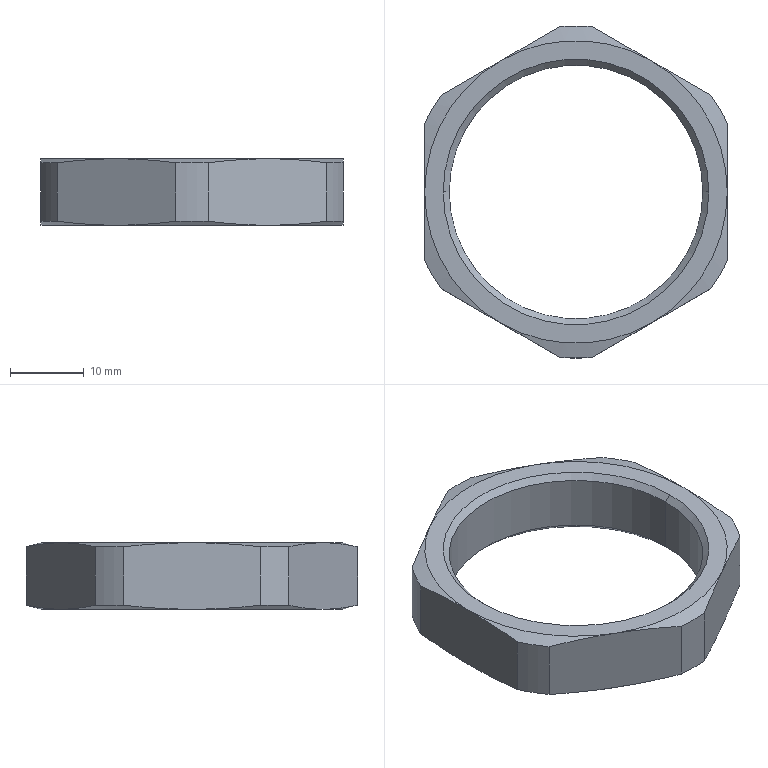Part | SolidWorks | features BaseBody 1 | 1 solid | 32 faces | box 41 x 45 x 9 mm | volume 4491 mm3 | cone 16 | cylinder 8 | plane 8 | commonest cylinder face diameters 45 x6 34.376 x2
STEP:
#1=CARTESIAN_POINT('',(-17.188,0.,0.812));
#2=VERTEX_POINT('',#1);
#3=CARTESIAN_POINT('',(17.188,0.,0.812));
#4=VERTEX_POINT('',#3);
#5=CARTESIAN_POINT('',(0.,0.,0.812));
#6=DIRECTION('',(0.,0.,1.));
#7=DIRECTION('',(1.,0.,0.));
#8=AXIS2_PLACEMENT_3D('',#5,#6,#7);
#9=CIRCLE('',#8,17.188);
#10=EDGE_CURVE('',#2,#4,#9,.T.);
#11=ORIENTED_EDGE('',*,*,#10,.F.);
#12=CARTESIAN_POINT('',(-17.188,0.,8.188));
#13=VERTEX_POINT('',#12);
#14=CARTESIAN_POINT('',(-17.188,0.,0.));
#15=DIRECTION('',(0.,0.,1.));
#16=VECTOR('',#15,1000.);
#17=LINE('',#14,#16);
#18=EDGE_CURVE('',#2,#13,#17,.T.);
#19=ORIENTED_EDGE('',*,*,#18,.T.);
#20=CARTESIAN_POINT('',(17.188,0.,8.188));
#21=VERTEX_POINT('',#20);
#22=CARTESIAN_POINT('',(0.,0.,8.188));
#23=DIRECTION('',(0.,0.,-1.));
#24=DIRECTION('',(1.,0.,0.));
#25=AXIS2_PLACEMENT_3D('',#22,#23,#24);
#26=CIRCLE('',#25,17.188);
#27=EDGE_CURVE('',#21,#13,#26,.T.);
#28=ORIENTED_EDGE('',*,*,#27,.F.);
#29=CARTESIAN_POINT('',(17.188,0.,0.));
#30=DIRECTION('',(0.,0.,1.));
#31=VECTOR('',#30,1000.);
#32=LINE('',#29,#31);
#33=EDGE_CURVE('',#4,#21,#32,.T.);
#34=ORIENTED_EDGE('',*,*,#33,.F.);
#35=EDGE_LOOP('',(#11,#19,#28,#34));
#36=FACE_OUTER_BOUND('',#35,.T.);
#37=CARTESIAN_POINT('',(0.,0.,0.));
#38=DIRECTION('',(0.,0.,1.));
#39=DIRECTION('',(1.,0.,0.));
#40=AXIS2_PLACEMENT_3D('',#37,#38,#39);
#41=CYLINDRICAL_SURFACE('',#40,17.188);
#42=ADVANCED_FACE('',(#36),#41,.F.);
#43=ORIENTED_EDGE('',*,*,#27,.T.);
#44=CARTESIAN_POINT('',(-18.,0.,9.));
#45=VERTEX_POINT('',#44);
#46=CARTESIAN_POINT('',(-18.,0.,9.));
#47=DIRECTION('',(-0.7071,0.,0.7071));
#48=VECTOR('',#47,1000.);
#49=LINE('',#46,#48);
#50=EDGE_CURVE('',#13,#45,#49,.T.);
#51=ORIENTED_EDGE('',*,*,#50,.T.);
#52=CARTESIAN_POINT('',(18.,0.,9.));
#53=VERTEX_POINT('',#52);
#54=CARTESIAN_POINT('',(0.,0.,9.));
#55=DIRECTION('',(0.,0.,-1.));
#56=DIRECTION('',(1.,0.,0.));
#57=AXIS2_PLACEMENT_3D('',#54,#55,#56);
#58=CIRCLE('',#57,18.);
#59=EDGE_CURVE('',#53,#45,#58,.T.);
#60=ORIENTED_EDGE('',*,*,#59,.F.);
#61=CARTESIAN_POINT('',(18.,0.,9.));
#62=DIRECTION('',(0.7071,0.,0.7071));
#63=VECTOR('',#62,1000.);
#64=LINE('',#61,#63);
#65=EDGE_CURVE('',#21,#53,#64,.T.);
#66=ORIENTED_EDGE('',*,*,#65,.F.);
#67=EDGE_LOOP('',(#43,#51,#60,#66));
#68=FACE_OUTER_BOUND('',#67,.T.);
#69=CARTESIAN_POINT('',(0.,0.,9.));
#70=DIRECTION('',(0.,0.,1.));
#71=DIRECTION('',(1.,0.,0.));
#72=AXIS2_PLACEMENT_3D('',#69,#70,#71);
#73=CONICAL_SURFACE('',#72,18.,0.7854);
#74=ADVANCED_FACE('',(#68),#73,.F.);
#75=ORIENTED_EDGE('',*,*,#10,.T.);
#76=CARTESIAN_POINT('',(18.,0.,0.));
#77=VERTEX_POINT('',#76);
#78=CARTESIAN_POINT('',(18.,0.,0.));
#79=DIRECTION('',(0.7071,0.,-0.7071));
#80=VECTOR('',#79,1000.);
#81=LINE('',#78,#80);
#82=EDGE_CURVE('',#4,#77,#81,.T.);
#83=ORIENTED_EDGE('',*,*,#82,.T.);
#84=CARTESIAN_POINT('',(-18.,0.,0.));
#85=VERTEX_POINT('',#84);
#86=CARTESIAN_POINT('',(0.,0.,0.));
#87=DIRECTION('',(0.,0.,1.));
#88=DIRECTION('',(-1.,0.,0.));
#89=AXIS2_PLACEMENT_3D('',#86,#87,#88);
#90=CIRCLE('',#89,18.);
#91=EDGE_CURVE('',#85,#77,#90,.T.);
#92=ORIENTED_EDGE('',*,*,#91,.F.);
#93=CARTESIAN_POINT('',(-18.,0.,0.));
#94=DIRECTION('',(-0.7071,0.,-0.7071));
#95=VECTOR('',#94,1000.);
#96=LINE('',#93,#95);
#97=EDGE_CURVE('',#2,#85,#96,.T.);
#98=ORIENTED_EDGE('',*,*,#97,.F.);
#99=EDGE_LOOP('',(#75,#83,#92,#98));
#100=FACE_OUTER_BOUND('',#99,.T.);
#101=CARTESIAN_POINT('',(0.,0.,0.));
#102=DIRECTION('',(0.,0.,-1.));
#103=DIRECTION('',(-1.,0.,0.));
#104=AXIS2_PLACEMENT_3D('',#101,#102,#103);
#105=CONICAL_SURFACE('',#104,18.,0.7854);
#106=ADVANCED_FACE('',(#100),#105,.F.);
#107=ORIENTED_EDGE('',*,*,#18,.F.);
#108=CARTESIAN_POINT('',(0.,0.,0.812));
#109=DIRECTION('',(0.,0.,1.));
#110=DIRECTION('',(1.,0.,0.));
#111=AXIS2_PLACEMENT_3D('',#108,#109,#110);
#112=CIRCLE('',#111,17.188);
#113=EDGE_CURVE('',#4,#2,#112,.T.);
#114=ORIENTED_EDGE('',*,*,#113,.F.);
#115=ORIENTED_EDGE('',*,*,#33,.T.);
#116=CARTESIAN_POINT('',(0.,0.,8.188));
#117=DIRECTION('',(0.,0.,-1.));
#118=DIRECTION('',(1.,0.,0.));
#119=AXIS2_PLACEMENT_3D('',#116,#117,#118);
#120=CIRCLE('',#119,17.188);
#121=EDGE_CURVE('',#13,#21,#120,.T.);
#122=ORIENTED_EDGE('',*,*,#121,.F.);
#123=EDGE_LOOP('',(#107,#114,#115,#122));
#124=FACE_OUTER_BOUND('',#123,.T.);
#125=CARTESIAN_POINT('',(0.,0.,0.));
#126=DIRECTION('',(0.,0.,1.));
#127=DIRECTION('',(1.,0.,0.));
#128=AXIS2_PLACEMENT_3D('',#125,#126,#127);
#129=CYLINDRICAL_SURFACE('',#128,17.188);
#130=ADVANCED_FACE('',(#124),#129,.F.);
#131=ORIENTED_EDGE('',*,*,#50,.F.);
#132=ORIENTED_EDGE('',*,*,#121,.T.);
#133=ORIENTED_EDGE('',*,*,#65,.T.);
#134=CARTESIAN_POINT('',(0.,0.,9.));
#135=DIRECTION('',(0.,0.,-1.));
#136=DIRECTION('',(1.,0.,0.));
#137=AXIS2_PLACEMENT_3D('',#134,#135,#136);
#138=CIRCLE('',#137,18.);
#139=EDGE_CURVE('',#45,#53,#138,.T.);
#140=ORIENTED_EDGE('',*,*,#139,.F.);
#141=EDGE_LOOP('',(#131,#132,#133,#140));
#142=FACE_OUTER_BOUND('',#141,.T.);
#143=CARTESIAN_POINT('',(0.,0.,9.));
#144=DIRECTION('',(0.,0.,1.));
#145=DIRECTION('',(1.,0.,0.));
#146=AXIS2_PLACEMENT_3D('',#143,#144,#145);
#147=CONICAL_SURFACE('',#146,18.,0.7854);
#148=ADVANCED_FACE('',(#142),#147,.F.);
#149=ORIENTED_EDGE('',*,*,#82,.F.);
#150=ORIENTED_EDGE('',*,*,#113,.T.);
#151=ORIENTED_EDGE('',*,*,#97,.T.);
#152=CARTESIAN_POINT('',(0.,0.,0.));
#153=DIRECTION('',(0.,0.,1.));
#154=DIRECTION('',(-1.,0.,0.));
#155=AXIS2_PLACEMENT_3D('',#152,#153,#154);
#156=CIRCLE('',#155,18.);
#157=EDGE_CURVE('',#77,#85,#156,.T.);
#158=ORIENTED_EDGE('',*,*,#157,.F.);
#159=EDGE_LOOP('',(#149,#150,#151,#158));
#160=FACE_OUTER_BOUND('',#159,.T.);
#161=CARTESIAN_POINT('',(0.,0.,0.));
#162=DIRECTION('',(0.,0.,-1.));
#163=DIRECTION('',(-1.,0.,0.));
#164=AXIS2_PLACEMENT_3D('',#161,#162,#163);
#165=CONICAL_SURFACE('',#164,18.,0.7854);
#166=ADVANCED_FACE('',(#160),#165,.F.);
#167=CARTESIAN_POINT('',(10.25,-17.754,9.));
#168=VERTEX_POINT('',#167);
#169=CARTESIAN_POINT('',(20.5,0.,9.));
#170=VERTEX_POINT('',#169);
#171=CARTESIAN_POINT('',(0.,0.,9.));
#172=DIRECTION('',(0.,0.,1.));
#173=DIRECTION('',(-1.,0.,0.));
#174=AXIS2_PLACEMENT_3D('',#171,#172,#173);
#175=CIRCLE('',#174,20.5);
#176=EDGE_CURVE('',#168,#170,#175,.T.);
#177=ORIENTED_EDGE('',*,*,#176,.T.);
#178=CARTESIAN_POINT('',(10.25,17.754,9.));
#179=VERTEX_POINT('',#178);
#180=CARTESIAN_POINT('',(0.,0.,9.));
#181=DIRECTION('',(0.,0.,1.));
#182=DIRECTION('',(-1.,0.,0.));
#183=AXIS2_PLACEMENT_3D('',#180,#181,#182);
#184=CIRCLE('',#183,20.5);
#185=EDGE_CURVE('',#170,#179,#184,.T.);
#186=ORIENTED_EDGE('',*,*,#185,.T.);
#187=CARTESIAN_POINT('',(-10.25,17.754,9.));
#188=VERTEX_POINT('',#187);
#189=CARTESIAN_POINT('',(0.,0.,9.));
#190=DIRECTION('',(0.,0.,1.));
#191=DIRECTION('',(-1.,0.,0.));
#192=AXIS2_PLACEMENT_3D('',#189,#190,#191);
#193=CIRCLE('',#192,20.5);
#194=EDGE_CURVE('',#179,#188,#193,.T.);
#195=ORIENTED_EDGE('',*,*,#194,.T.);
#196=CARTESIAN_POINT('',(-20.5,0.,9.));
#197=VERTEX_POINT('',#196);
#198=CARTESIAN_POINT('',(0.,0.,9.));
#199=DIRECTION('',(0.,0.,1.));
#200=DIRECTION('',(-1.,0.,0.));
#201=AXIS2_PLACEMENT_3D('',#198,#199,#200);
#202=CIRCLE('',#201,20.5);
#203=EDGE_CURVE('',#188,#197,#202,.T.);
#204=ORIENTED_EDGE('',*,*,#203,.T.);
#205=CARTESIAN_POINT('',(-10.25,-17.754,9.));
#206=VERTEX_POINT('',#205);
#207=CARTESIAN_POINT('',(0.,0.,9.));
#208=DIRECTION('',(0.,0.,1.));
#209=DIRECTION('',(-1.,0.,0.));
#210=AXIS2_PLACEMENT_3D('',#207,#208,#209);
#211=CIRCLE('',#210,20.5);
#212=EDGE_CURVE('',#197,#206,#211,.T.);
#213=ORIENTED_EDGE('',*,*,#212,.T.);
#214=CARTESIAN_POINT('',(0.,0.,9.));
#215=DIRECTION('',(0.,0.,1.));
#216=DIRECTION('',(-1.,0.,0.));
#217=AXIS2_PLACEMENT_3D('',#214,#215,#216);
#218=CIRCLE('',#217,20.5);
#219=EDGE_CURVE('',#206,#168,#218,.T.);
#220=ORIENTED_EDGE('',*,*,#219,.T.);
#221=EDGE_LOOP('',(#177,#186,#195,#204,#213,#220));
#222=FACE_OUTER_BOUND('',#221,.T.);
#223=ORIENTED_EDGE('',*,*,#59,.T.);
#224=ORIENTED_EDGE('',*,*,#139,.T.);
#225=EDGE_LOOP('',(#223,#224));
#226=FACE_BOUND('',#225,.T.);
#227=CARTESIAN_POINT('',(0.,20.5,9.));
#228=DIRECTION('',(0.,0.,1.));
#229=DIRECTION('',(1.,0.,0.));
#230=AXIS2_PLACEMENT_3D('',#227,#228,#229);
#231=PLANE('',#230);
#232=ADVANCED_FACE('',(#222,#226),#231,.T.);
#233=ORIENTED_EDGE('',*,*,#91,.T.);
#234=ORIENTED_EDGE('',*,*,#157,.T.);
#235=EDGE_LOOP('',(#233,#234));
#236=FACE_BOUND('',#235,.T.);
#237=CARTESIAN_POINT('',(10.25,-17.754,0.));
#238=VERTEX_POINT('',#237);
#239=CARTESIAN_POINT('',(-10.25,-17.754,0.));
#240=VERTEX_POINT('',#239);
#241=CARTESIAN_POINT('',(0.,0.,0.));
#242=DIRECTION('',(0.,0.,-1.));
#243=DIRECTION('',(1.,0.,0.));
#244=AXIS2_PLACEMENT_3D('',#241,#242,#243);
#245=CIRCLE('',#244,20.5);
#246=EDGE_CURVE('',#238,#240,#245,.T.);
#247=ORIENTED_EDGE('',*,*,#246,.T.);
#248=CARTESIAN_POINT('',(-20.5,0.,0.));
#249=VERTEX_POINT('',#248);
#250=CARTESIAN_POINT('',(0.,0.,0.));
#251=DIRECTION('',(0.,0.,-1.));
#252=DIRECTION('',(1.,0.,0.));
#253=AXIS2_PLACEMENT_3D('',#250,#251,#252);
#254=CIRCLE('',#253,20.5);
#255=EDGE_CURVE('',#240,#249,#254,.T.);
#256=ORIENTED_EDGE('',*,*,#255,.T.);
#257=CARTESIAN_POINT('',(-10.25,17.754,0.));
#258=VERTEX_POINT('',#257);
#259=CARTESIAN_POINT('',(0.,0.,0.));
#260=DIRECTION('',(0.,0.,-1.));
#261=DIRECTION('',(1.,0.,0.));
#262=AXIS2_PLACEMENT_3D('',#259,#260,#261);
#263=CIRCLE('',#262,20.5);
#264=EDGE_CURVE('',#249,#258,#263,.T.);
#265=ORIENTED_EDGE('',*,*,#264,.T.);
#266=CARTESIAN_POINT('',(10.25,17.754,0.));
#267=VERTEX_POINT('',#266);
#268=CARTESIAN_POINT('',(0.,0.,0.));
#269=DIRECTION('',(0.,0.,-1.));
#270=DIRECTION('',(1.,0.,0.));
#271=AXIS2_PLACEMENT_3D('',#268,#269,#270);
#272=CIRCLE('',#271,20.5);
#273=EDGE_CURVE('',#258,#267,#272,.T.);
#274=ORIENTED_EDGE('',*,*,#273,.T.);
#275=CARTESIAN_POINT('',(20.5,0.,0.));
#276=VERTEX_POINT('',#275);
#277=CARTESIAN_POINT('',(0.,0.,0.));
#278=DIRECTION('',(0.,0.,-1.));
#279=DIRECTION('',(1.,0.,0.));
#280=AXIS2_PLACEMENT_3D('',#277,#278,#279);
#281=CIRCLE('',#280,20.5);
#282=EDGE_CURVE('',#267,#276,#281,.T.);
#283=ORIENTED_EDGE('',*,*,#282,.T.);
#284=CARTESIAN_POINT('',(0.,0.,0.));
#285=DIRECTION('',(0.,0.,-1.));
#286=DIRECTION('',(1.,0.,0.));
#287=AXIS2_PLACEMENT_3D('',#284,#285,#286);
#288=CIRCLE('',#287,20.5);
#289=EDGE_CURVE('',#276,#238,#288,.T.);
#290=ORIENTED_EDGE('',*,*,#289,.T.);
#291=EDGE_LOOP('',(#247,#256,#265,#274,#283,#290));
#292=FACE_OUTER_BOUND('',#291,.T.);
#293=CARTESIAN_POINT('',(0.,18.,0.));
#294=DIRECTION('',(0.,0.,-1.));
#295=DIRECTION('',(-1.,0.,0.));
#296=AXIS2_PLACEMENT_3D('',#293,#294,#295);
#297=PLANE('',#296);
#298=ADVANCED_FACE('',(#236,#292),#297,.T.);
#299=CARTESIAN_POINT('',(20.5,9.274,8.464));
#300=VERTEX_POINT('',#299);
#301=CARTESIAN_POINT('',(20.5,0.,9.));
#302=CARTESIAN_POINT('',(20.5,1.551,9.));
#303=CARTESIAN_POINT('',(20.5,3.099,8.952));
#304=CARTESIAN_POINT('',(20.5,6.19,8.769));
#305=CARTESIAN_POINT('',(20.5,7.733,8.634));
#306=CARTESIAN_POINT('',(20.5,9.274,8.464));
#307=B_SPLINE_CURVE_WITH_KNOTS('',3,(#301,#302,#303,#304,#305,#306),.UNSPECIFIED.,.F.,.F.,(4,2,4),(0.,0.004645,0.009289),.UNSPECIFIED.);
#308=EDGE_CURVE('',#170,#300,#307,.T.);
#309=ORIENTED_EDGE('',*,*,#308,.T.);
#310=CARTESIAN_POINT('',(18.281,13.117,8.464));
#311=VERTEX_POINT('',#310);
#312=CARTESIAN_POINT('',(0.,0.,8.464));
#313=DIRECTION('',(0.,0.,1.));
#314=DIRECTION('',(-1.,0.,0.));
#315=AXIS2_PLACEMENT_3D('',#312,#313,#314);
#316=CIRCLE('',#315,22.5);
#317=EDGE_CURVE('',#300,#311,#316,.T.);
#318=ORIENTED_EDGE('',*,*,#317,.T.);
#319=CARTESIAN_POINT('',(18.281,13.117,8.464));
#320=CARTESIAN_POINT('',(16.947,13.887,8.634));
#321=CARTESIAN_POINT('',(15.61,14.659,8.769));
#322=CARTESIAN_POINT('',(12.934,16.204,8.952));
#323=CARTESIAN_POINT('',(11.593,16.978,9.));
#324=CARTESIAN_POINT('',(10.25,17.754,9.));
#325=B_SPLINE_CURVE_WITH_KNOTS('',3,(#319,#320,#321,#322,#323,#324),.UNSPECIFIED.,.F.,.F.,(4,2,4),(0.,0.004645,0.009289),.UNSPECIFIED.);
#326=EDGE_CURVE('',#311,#179,#325,.T.);
#327=ORIENTED_EDGE('',*,*,#326,.T.);
#328=ORIENTED_EDGE('',*,*,#185,.F.);
#329=EDGE_LOOP('',(#309,#318,#327,#328));
#330=FACE_OUTER_BOUND('',#329,.T.);
#331=CARTESIAN_POINT('',(0.,0.,8.464));
#332=DIRECTION('',(0.,0.,-1.));
#333=DIRECTION('',(-1.,0.,0.));
#334=AXIS2_PLACEMENT_3D('',#331,#332,#333);
#335=CONICAL_SURFACE('',#334,22.5,1.309);
#336=ADVANCED_FACE('',(#330),#335,.T.);
#337=CARTESIAN_POINT('',(18.281,-13.117,8.464));
#338=VERTEX_POINT('',#337);
#339=CARTESIAN_POINT('',(10.25,-17.754,9.));
#340=CARTESIAN_POINT('',(11.593,-16.978,9.));
#341=CARTESIAN_POINT('',(12.934,-16.204,8.952));
#342=CARTESIAN_POINT('',(15.61,-14.659,8.769));
#343=CARTESIAN_POINT('',(16.947,-13.887,8.634));
#344=CARTESIAN_POINT('',(18.281,-13.117,8.464));
#345=B_SPLINE_CURVE_WITH_KNOTS('',3,(#339,#340,#341,#342,#343,#344),.UNSPECIFIED.,.F.,.F.,(4,2,4),(0.,0.004645,0.009289),.UNSPECIFIED.);
#346=EDGE_CURVE('',#168,#338,#345,.T.);
#347=ORIENTED_EDGE('',*,*,#346,.T.);
#348=CARTESIAN_POINT('',(20.5,-9.274,8.464));
#349=VERTEX_POINT('',#348);
#350=CARTESIAN_POINT('',(0.,0.,8.464));
#351=DIRECTION('',(0.,0.,1.));
#352=DIRECTION('',(-1.,0.,0.));
#353=AXIS2_PLACEMENT_3D('',#350,#351,#352);
#354=CIRCLE('',#353,22.5);
#355=EDGE_CURVE('',#338,#349,#354,.T.);
#356=ORIENTED_EDGE('',*,*,#355,.T.);
#357=CARTESIAN_POINT('',(20.5,-9.274,8.464));
#358=CARTESIAN_POINT('',(20.5,-7.733,8.634));
#359=CARTESIAN_POINT('',(20.5,-6.19,8.769));
#360=CARTESIAN_POINT('',(20.5,-3.099,8.952));
#361=CARTESIAN_POINT('',(20.5,-1.551,9.));
#362=CARTESIAN_POINT('',(20.5,0.,9.));
#363=B_SPLINE_CURVE_WITH_KNOTS('',3,(#357,#358,#359,#360,#361,#362),.UNSPECIFIED.,.F.,.F.,(4,2,4),(0.,0.004645,0.009289),.UNSPECIFIED.);
#364=EDGE_CURVE('',#349,#170,#363,.T.);
#365=ORIENTED_EDGE('',*,*,#364,.T.);
#366=ORIENTED_EDGE('',*,*,#176,.F.);
#367=EDGE_LOOP('',(#347,#356,#365,#366));
#368=FACE_OUTER_BOUND('',#367,.T.);
#369=CARTESIAN_POINT('',(0.,0.,8.464));
#370=DIRECTION('',(0.,0.,-1.));
#371=DIRECTION('',(-1.,0.,0.));
#372=AXIS2_PLACEMENT_3D('',#369,#370,#371);
#373=CONICAL_SURFACE('',#372,22.5,1.309);
#374=ADVANCED_FACE('',(#368),#373,.T.);
#375=CARTESIAN_POINT('',(-2.219,-22.39,8.464));
#376=VERTEX_POINT('',#375);
#377=CARTESIAN_POINT('',(-10.25,-17.754,9.));
#378=CARTESIAN_POINT('',(-8.907,-18.529,9.));
#379=CARTESIAN_POINT('',(-7.566,-19.303,8.952));
#380=CARTESIAN_POINT('',(-4.89,-20.848,8.769));
#381=CARTESIAN_POINT('',(-3.553,-21.62,8.634));
#382=CARTESIAN_POINT('',(-2.219,-22.39,8.464));
#383=B_SPLINE_CURVE_WITH_KNOTS('',3,(#377,#378,#379,#380,#381,#382),.UNSPECIFIED.,.F.,.F.,(4,2,4),(0.,0.004645,0.009289),.UNSPECIFIED.);
#384=EDGE_CURVE('',#206,#376,#383,.T.);
#385=ORIENTED_EDGE('',*,*,#384,.T.);
#386=CARTESIAN_POINT('',(2.219,-22.39,8.464));
#387=VERTEX_POINT('',#386);
#388=CARTESIAN_POINT('',(0.,0.,8.464));
#389=DIRECTION('',(0.,0.,1.));
#390=DIRECTION('',(-1.,0.,0.));
#391=AXIS2_PLACEMENT_3D('',#388,#389,#390);
#392=CIRCLE('',#391,22.5);
#393=EDGE_CURVE('',#376,#387,#392,.T.);
#394=ORIENTED_EDGE('',*,*,#393,.T.);
#395=CARTESIAN_POINT('',(2.219,-22.39,8.464));
#396=CARTESIAN_POINT('',(3.553,-21.62,8.634));
#397=CARTESIAN_POINT('',(4.89,-20.848,8.769));
#398=CARTESIAN_POINT('',(7.566,-19.303,8.952));
#399=CARTESIAN_POINT('',(8.907,-18.529,9.));
#400=CARTESIAN_POINT('',(10.25,-17.754,9.));
#401=B_SPLINE_CURVE_WITH_KNOTS('',3,(#395,#396,#397,#398,#399,#400),.UNSPECIFIED.,.F.,.F.,(4,2,4),(0.,0.004645,0.009289),.UNSPECIFIED.);
#402=EDGE_CURVE('',#387,#168,#401,.T.);
#403=ORIENTED_EDGE('',*,*,#402,.T.);
#404=ORIENTED_EDGE('',*,*,#219,.F.);
#405=EDGE_LOOP('',(#385,#394,#403,#404));
#406=FACE_OUTER_BOUND('',#405,.T.);
#407=CARTESIAN_POINT('',(0.,0.,8.464));
#408=DIRECTION('',(0.,0.,-1.));
#409=DIRECTION('',(-1.,0.,0.));
#410=AXIS2_PLACEMENT_3D('',#407,#408,#409);
#411=CONICAL_SURFACE('',#410,22.5,1.309);
#412=ADVANCED_FACE('',(#406),#411,.T.);
#413=CARTESIAN_POINT('',(-18.281,-13.117,8.464));
#414=VERTEX_POINT('',#413);
#415=CARTESIAN_POINT('',(-18.281,-13.117,8.464));
#416=CARTESIAN_POINT('',(-16.947,-13.887,8.634));
#417=CARTESIAN_POINT('',(-15.61,-14.659,8.769));
#418=CARTESIAN_POINT('',(-12.934,-16.204,8.952));
#419=CARTESIAN_POINT('',(-11.593,-16.978,9.));
#420=CARTESIAN_POINT('',(-10.25,-17.754,9.));
#421=B_SPLINE_CURVE_WITH_KNOTS('',3,(#415,#416,#417,#418,#419,#420),.UNSPECIFIED.,.F.,.F.,(4,2,4),(0.,0.004645,0.009289),.UNSPECIFIED.);
#422=EDGE_CURVE('',#414,#206,#421,.T.);
#423=ORIENTED_EDGE('',*,*,#422,.T.);
#424=ORIENTED_EDGE('',*,*,#212,.F.);
#425=CARTESIAN_POINT('',(-20.5,-9.274,8.464));
#426=VERTEX_POINT('',#425);
#427=CARTESIAN_POINT('',(-20.5,0.,9.));
#428=CARTESIAN_POINT('',(-20.5,-1.551,9.));
#429=CARTESIAN_POINT('',(-20.5,-3.099,8.952));
#430=CARTESIAN_POINT('',(-20.5,-6.19,8.769));
#431=CARTESIAN_POINT('',(-20.5,-7.733,8.634));
#432=CARTESIAN_POINT('',(-20.5,-9.274,8.464));
#433=B_SPLINE_CURVE_WITH_KNOTS('',3,(#427,#428,#429,#430,#431,#432),.UNSPECIFIED.,.F.,.F.,(4,2,4),(0.,0.004645,0.009289),.UNSPECIFIED.);
#434=EDGE_CURVE('',#197,#426,#433,.T.);
#435=ORIENTED_EDGE('',*,*,#434,.T.);
#436=CARTESIAN_POINT('',(0.,0.,8.464));
#437=DIRECTION('',(0.,0.,1.));
#438=DIRECTION('',(-1.,0.,0.));
#439=AXIS2_PLACEMENT_3D('',#436,#437,#438);
#440=CIRCLE('',#439,22.5);
#441=EDGE_CURVE('',#426,#414,#440,.T.);
#442=ORIENTED_EDGE('',*,*,#441,.T.);
#443=EDGE_LOOP('',(#423,#424,#435,#442));
#444=FACE_OUTER_BOUND('',#443,.T.);
#445=CARTESIAN_POINT('',(0.,0.,8.464));
#446=DIRECTION('',(0.,0.,-1.));
#447=DIRECTION('',(-1.,0.,0.));
#448=AXIS2_PLACEMENT_3D('',#445,#446,#447);
#449=CONICAL_SURFACE('',#448,22.5,1.309);
#450=ADVANCED_FACE('',(#444),#449,.T.);
#451=CARTESIAN_POINT('',(-18.281,13.117,8.464));
#452=VERTEX_POINT('',#451);
#453=CARTESIAN_POINT('',(-10.25,17.754,9.));
#454=CARTESIAN_POINT('',(-11.593,16.978,9.));
#455=CARTESIAN_POINT('',(-12.934,16.204,8.952));
#456=CARTESIAN_POINT('',(-15.61,14.659,8.769));
#457=CARTESIAN_POINT('',(-16.947,13.887,8.634));
#458=CARTESIAN_POINT('',(-18.281,13.117,8.464));
#459=B_SPLINE_CURVE_WITH_KNOTS('',3,(#453,#454,#455,#456,#457,#458),.UNSPECIFIED.,.F.,.F.,(4,2,4),(0.,0.004645,0.009289),.UNSPECIFIED.);
#460=EDGE_CURVE('',#188,#452,#459,.T.);
#461=ORIENTED_EDGE('',*,*,#460,.T.);
#462=CARTESIAN_POINT('',(-20.5,9.274,8.464));
#463=VERTEX_POINT('',#462);
#464=CARTESIAN_POINT('',(0.,0.,8.464));
#465=DIRECTION('',(0.,0.,1.));
#466=DIRECTION('',(-1.,0.,0.));
#467=AXIS2_PLACEMENT_3D('',#464,#465,#466);
#468=CIRCLE('',#467,22.5);
#469=EDGE_CURVE('',#452,#463,#468,.T.);
#470=ORIENTED_EDGE('',*,*,#469,.T.);
#471=CARTESIAN_POINT('',(-20.5,9.274,8.464));
#472=CARTESIAN_POINT('',(-20.5,7.733,8.634));
#473=CARTESIAN_POINT('',(-20.5,6.19,8.769));
#474=CARTESIAN_POINT('',(-20.5,3.099,8.952));
#475=CARTESIAN_POINT('',(-20.5,1.551,9.));
#476=CARTESIAN_POINT('',(-20.5,0.,9.));
#477=B_SPLINE_CURVE_WITH_KNOTS('',3,(#471,#472,#473,#474,#475,#476),.UNSPECIFIED.,.F.,.F.,(4,2,4),(0.,0.004645,0.009289),.UNSPECIFIED.);
#478=EDGE_CURVE('',#463,#197,#477,.T.);
#479=ORIENTED_EDGE('',*,*,#478,.T.);
#480=ORIENTED_EDGE('',*,*,#203,.F.);
#481=EDGE_LOOP('',(#461,#470,#479,#480));
#482=FACE_OUTER_BOUND('',#481,.T.);
#483=CARTESIAN_POINT('',(0.,0.,8.464));
#484=DIRECTION('',(0.,0.,-1.));
#485=DIRECTION('',(-1.,0.,0.));
#486=AXIS2_PLACEMENT_3D('',#483,#484,#485);
#487=CONICAL_SURFACE('',#486,22.5,1.309);
#488=ADVANCED_FACE('',(#482),#487,.T.);
#489=CARTESIAN_POINT('',(2.219,22.39,8.464));
#490=VERTEX_POINT('',#489);
#491=CARTESIAN_POINT('',(10.25,17.754,9.));
#492=CARTESIAN_POINT('',(8.907,18.529,9.));
#493=CARTESIAN_POINT('',(7.566,19.303,8.952));
#494=CARTESIAN_POINT('',(4.89,20.848,8.769));
#495=CARTESIAN_POINT('',(3.553,21.62,8.634));
#496=CARTESIAN_POINT('',(2.219,22.39,8.464));
#497=B_SPLINE_CURVE_WITH_KNOTS('',3,(#491,#492,#493,#494,#495,#496),.UNSPECIFIED.,.F.,.F.,(4,2,4),(0.,0.004645,0.009289),.UNSPECIFIED.);
#498=EDGE_CURVE('',#179,#490,#497,.T.);
#499=ORIENTED_EDGE('',*,*,#498,.T.);
#500=CARTESIAN_POINT('',(-2.219,22.39,8.464));
#501=VERTEX_POINT('',#500);
#502=CARTESIAN_POINT('',(0.,0.,8.464));
#503=DIRECTION('',(0.,0.,1.));
#504=DIRECTION('',(-1.,0.,0.));
#505=AXIS2_PLACEMENT_3D('',#502,#503,#504);
#506=CIRCLE('',#505,22.5);
#507=EDGE_CURVE('',#490,#501,#506,.T.);
#508=ORIENTED_EDGE('',*,*,#507,.T.);
#509=CARTESIAN_POINT('',(-2.219,22.39,8.464));
#510=CARTESIAN_POINT('',(-3.553,21.62,8.634));
#511=CARTESIAN_POINT('',(-4.89,20.848,8.769));
#512=CARTESIAN_POINT('',(-7.566,19.303,8.952));
#513=CARTESIAN_POINT('',(-8.907,18.529,9.));
#514=CARTESIAN_POINT('',(-10.25,17.754,9.));
#515=B_SPLINE_CURVE_WITH_KNOTS('',3,(#509,#510,#511,#512,#513,#514),.UNSPECIFIED.,.F.,.F.,(4,2,4),(0.,0.004645,0.009289),.UNSPECIFIED.);
#516=EDGE_CURVE('',#501,#188,#515,.T.);
#517=ORIENTED_EDGE('',*,*,#516,.T.);
#518=ORIENTED_EDGE('',*,*,#194,.F.);
#519=EDGE_LOOP('',(#499,#508,#517,#518));
#520=FACE_OUTER_BOUND('',#519,.T.);
#521=CARTESIAN_POINT('',(0.,0.,8.464));
#522=DIRECTION('',(0.,0.,-1.));
#523=DIRECTION('',(-1.,0.,0.));
#524=AXIS2_PLACEMENT_3D('',#521,#522,#523);
#525=CONICAL_SURFACE('',#524,22.5,1.309);
#526=ADVANCED_FACE('',(#520),#525,.T.);
#527=CARTESIAN_POINT('',(-18.281,-13.117,0.5359));
#528=VERTEX_POINT('',#527);
#529=CARTESIAN_POINT('',(-10.25,-17.754,0.));
#530=CARTESIAN_POINT('',(-11.593,-16.978,0.));
#531=CARTESIAN_POINT('',(-12.934,-16.204,0.0477));
#532=CARTESIAN_POINT('',(-15.61,-14.659,0.2307));
#533=CARTESIAN_POINT('',(-16.947,-13.887,0.3657));
#534=CARTESIAN_POINT('',(-18.281,-13.117,0.5359));
#535=B_SPLINE_CURVE_WITH_KNOTS('',3,(#529,#530,#531,#532,#533,#534),.UNSPECIFIED.,.F.,.F.,(4,2,4),(0.,0.004645,0.009289),.UNSPECIFIED.);
#536=EDGE_CURVE('',#240,#528,#535,.T.);
#537=ORIENTED_EDGE('',*,*,#536,.T.);
#538=CARTESIAN_POINT('',(-20.5,-9.274,0.5359));
#539=VERTEX_POINT('',#538);
#540=CARTESIAN_POINT('',(0.,0.,0.5359));
#541=DIRECTION('',(0.,0.,-1.));
#542=DIRECTION('',(1.,0.,0.));
#543=AXIS2_PLACEMENT_3D('',#540,#541,#542);
#544=CIRCLE('',#543,22.5);
#545=EDGE_CURVE('',#528,#539,#544,.T.);
#546=ORIENTED_EDGE('',*,*,#545,.T.);
#547=CARTESIAN_POINT('',(-20.5,-9.274,0.5359));
#548=CARTESIAN_POINT('',(-20.5,-7.733,0.3657));
#549=CARTESIAN_POINT('',(-20.5,-6.19,0.2307));
#550=CARTESIAN_POINT('',(-20.5,-3.099,0.0477));
#551=CARTESIAN_POINT('',(-20.5,-1.551,0.));
#552=CARTESIAN_POINT('',(-20.5,0.,0.));
#553=B_SPLINE_CURVE_WITH_KNOTS('',3,(#547,#548,#549,#550,#551,#552),.UNSPECIFIED.,.F.,.F.,(4,2,4),(0.,0.004645,0.009289),.UNSPECIFIED.);
#554=EDGE_CURVE('',#539,#249,#553,.T.);
#555=ORIENTED_EDGE('',*,*,#554,.T.);
#556=ORIENTED_EDGE('',*,*,#255,.F.);
#557=EDGE_LOOP('',(#537,#546,#555,#556));
#558=FACE_OUTER_BOUND('',#557,.T.);
#559=CARTESIAN_POINT('',(0.,0.,0.5359));
#560=DIRECTION('',(0.,0.,1.));
#561=DIRECTION('',(1.,0.,0.));
#562=AXIS2_PLACEMENT_3D('',#559,#560,#561);
#563=CONICAL_SURFACE('',#562,22.5,1.309);
#564=ADVANCED_FACE('',(#558),#563,.T.);
#565=CARTESIAN_POINT('',(-2.219,-22.39,0.5359));
#566=VERTEX_POINT('',#565);
#567=CARTESIAN_POINT('',(-2.219,-22.39,0.5359));
#568=CARTESIAN_POINT('',(-3.553,-21.62,0.3657));
#569=CARTESIAN_POINT('',(-4.89,-20.848,0.2307));
#570=CARTESIAN_POINT('',(-7.566,-19.303,0.0477));
#571=CARTESIAN_POINT('',(-8.907,-18.529,0.));
#572=CARTESIAN_POINT('',(-10.25,-17.754,0.));
#573=B_SPLINE_CURVE_WITH_KNOTS('',3,(#567,#568,#569,#570,#571,#572),.UNSPECIFIED.,.F.,.F.,(4,2,4),(0.,0.004645,0.009289),.UNSPECIFIED.);
#574=EDGE_CURVE('',#566,#240,#573,.T.);
#575=ORIENTED_EDGE('',*,*,#574,.T.);
#576=ORIENTED_EDGE('',*,*,#246,.F.);
#577=CARTESIAN_POINT('',(2.219,-22.39,0.5359));
#578=VERTEX_POINT('',#577);
#579=CARTESIAN_POINT('',(10.25,-17.754,0.));
#580=CARTESIAN_POINT('',(8.907,-18.529,0.));
#581=CARTESIAN_POINT('',(7.566,-19.303,0.0477));
#582=CARTESIAN_POINT('',(4.89,-20.848,0.2307));
#583=CARTESIAN_POINT('',(3.553,-21.62,0.3657));
#584=CARTESIAN_POINT('',(2.219,-22.39,0.5359));
#585=B_SPLINE_CURVE_WITH_KNOTS('',3,(#579,#580,#581,#582,#583,#584),.UNSPECIFIED.,.F.,.F.,(4,2,4),(0.,0.004645,0.009289),.UNSPECIFIED.);
#586=EDGE_CURVE('',#238,#578,#585,.T.);
#587=ORIENTED_EDGE('',*,*,#586,.T.);
#588=CARTESIAN_POINT('',(0.,0.,0.5359));
#589=DIRECTION('',(0.,0.,-1.));
#590=DIRECTION('',(1.,0.,0.));
#591=AXIS2_PLACEMENT_3D('',#588,#589,#590);
#592=CIRCLE('',#591,22.5);
#593=EDGE_CURVE('',#578,#566,#592,.T.);
#594=ORIENTED_EDGE('',*,*,#593,.T.);
#595=EDGE_LOOP('',(#575,#576,#587,#594));
#596=FACE_OUTER_BOUND('',#595,.T.);
#597=CARTESIAN_POINT('',(0.,0.,0.5359));
#598=DIRECTION('',(0.,0.,1.));
#599=DIRECTION('',(1.,0.,0.));
#600=AXIS2_PLACEMENT_3D('',#597,#598,#599);
#601=CONICAL_SURFACE('',#600,22.5,1.309);
#602=ADVANCED_FACE('',(#596),#601,.T.);
#603=CARTESIAN_POINT('',(18.281,-13.117,0.5359));
#604=VERTEX_POINT('',#603);
#605=CARTESIAN_POINT('',(18.281,-13.117,0.5359));
#606=CARTESIAN_POINT('',(16.947,-13.887,0.3657));
#607=CARTESIAN_POINT('',(15.61,-14.659,0.2307));
#608=CARTESIAN_POINT('',(12.934,-16.204,0.0477));
#609=CARTESIAN_POINT('',(11.593,-16.978,0.));
#610=CARTESIAN_POINT('',(10.25,-17.754,0.));
#611=B_SPLINE_CURVE_WITH_KNOTS('',3,(#605,#606,#607,#608,#609,#610),.UNSPECIFIED.,.F.,.F.,(4,2,4),(0.,0.004645,0.009289),.UNSPECIFIED.);
#612=EDGE_CURVE('',#604,#238,#611,.T.);
#613=ORIENTED_EDGE('',*,*,#612,.T.);
#614=ORIENTED_EDGE('',*,*,#289,.F.);
#615=CARTESIAN_POINT('',(20.5,-9.274,0.5359));
#616=VERTEX_POINT('',#615);
#617=CARTESIAN_POINT('',(20.5,0.,0.));
#618=CARTESIAN_POINT('',(20.5,-1.551,0.));
#619=CARTESIAN_POINT('',(20.5,-3.099,0.0477));
#620=CARTESIAN_POINT('',(20.5,-6.19,0.2307));
#621=CARTESIAN_POINT('',(20.5,-7.733,0.3657));
#622=CARTESIAN_POINT('',(20.5,-9.274,0.5359));
#623=B_SPLINE_CURVE_WITH_KNOTS('',3,(#617,#618,#619,#620,#621,#622),.UNSPECIFIED.,.F.,.F.,(4,2,4),(0.,0.004645,0.009289),.UNSPECIFIED.);
#624=EDGE_CURVE('',#276,#616,#623,.T.);
#625=ORIENTED_EDGE('',*,*,#624,.T.);
#626=CARTESIAN_POINT('',(0.,0.,0.5359));
#627=DIRECTION('',(0.,0.,-1.));
#628=DIRECTION('',(1.,0.,0.));
#629=AXIS2_PLACEMENT_3D('',#626,#627,#628);
#630=CIRCLE('',#629,22.5);
#631=EDGE_CURVE('',#616,#604,#630,.T.);
#632=ORIENTED_EDGE('',*,*,#631,.T.);
#633=EDGE_LOOP('',(#613,#614,#625,#632));
#634=FACE_OUTER_BOUND('',#633,.T.);
#635=CARTESIAN_POINT('',(0.,0.,0.5359));
#636=DIRECTION('',(0.,0.,1.));
#637=DIRECTION('',(1.,0.,0.));
#638=AXIS2_PLACEMENT_3D('',#635,#636,#637);
#639=CONICAL_SURFACE('',#638,22.5,1.309);
#640=ADVANCED_FACE('',(#634),#639,.T.);
#641=CARTESIAN_POINT('',(20.5,9.274,0.5359));
#642=VERTEX_POINT('',#641);
#643=CARTESIAN_POINT('',(20.5,9.274,0.5359));
#644=CARTESIAN_POINT('',(20.5,7.733,0.3657));
#645=CARTESIAN_POINT('',(20.5,6.19,0.2307));
#646=CARTESIAN_POINT('',(20.5,3.099,0.0477));
#647=CARTESIAN_POINT('',(20.5,1.551,0.));
#648=CARTESIAN_POINT('',(20.5,0.,0.));
#649=B_SPLINE_CURVE_WITH_KNOTS('',3,(#643,#644,#645,#646,#647,#648),.UNSPECIFIED.,.F.,.F.,(4,2,4),(0.,0.004645,0.009289),.UNSPECIFIED.);
#650=EDGE_CURVE('',#642,#276,#649,.T.);
#651=ORIENTED_EDGE('',*,*,#650,.T.);
#652=ORIENTED_EDGE('',*,*,#282,.F.);
#653=CARTESIAN_POINT('',(18.281,13.117,0.5359));
#654=VERTEX_POINT('',#653);
#655=CARTESIAN_POINT('',(10.25,17.754,0.));
#656=CARTESIAN_POINT('',(11.593,16.978,0.));
#657=CARTESIAN_POINT('',(12.934,16.204,0.0477));
#658=CARTESIAN_POINT('',(15.61,14.659,0.2307));
#659=CARTESIAN_POINT('',(16.947,13.887,0.3657));
#660=CARTESIAN_POINT('',(18.281,13.117,0.5359));
#661=B_SPLINE_CURVE_WITH_KNOTS('',3,(#655,#656,#657,#658,#659,#660),.UNSPECIFIED.,.F.,.F.,(4,2,4),(0.,0.004645,0.009289),.UNSPECIFIED.);
#662=EDGE_CURVE('',#267,#654,#661,.T.);
#663=ORIENTED_EDGE('',*,*,#662,.T.);
#664=CARTESIAN_POINT('',(0.,0.,0.5359));
#665=DIRECTION('',(0.,0.,-1.));
#666=DIRECTION('',(1.,0.,0.));
#667=AXIS2_PLACEMENT_3D('',#664,#665,#666);
#668=CIRCLE('',#667,22.5);
#669=EDGE_CURVE('',#654,#642,#668,.T.);
#670=ORIENTED_EDGE('',*,*,#669,.T.);
#671=EDGE_LOOP('',(#651,#652,#663,#670));
#672=FACE_OUTER_BOUND('',#671,.T.);
#673=CARTESIAN_POINT('',(0.,0.,0.5359));
#674=DIRECTION('',(0.,0.,1.));
#675=DIRECTION('',(1.,0.,0.));
#676=AXIS2_PLACEMENT_3D('',#673,#674,#675);
#677=CONICAL_SURFACE('',#676,22.5,1.309);
#678=ADVANCED_FACE('',(#672),#677,.T.);
#679=CARTESIAN_POINT('',(-2.219,22.39,0.5359));
#680=VERTEX_POINT('',#679);
#681=CARTESIAN_POINT('',(-10.25,17.754,0.));
#682=CARTESIAN_POINT('',(-8.907,18.529,0.));
#683=CARTESIAN_POINT('',(-7.566,19.303,0.0477));
#684=CARTESIAN_POINT('',(-4.89,20.848,0.2307));
#685=CARTESIAN_POINT('',(-3.553,21.62,0.3657));
#686=CARTESIAN_POINT('',(-2.219,22.39,0.5359));
#687=B_SPLINE_CURVE_WITH_KNOTS('',3,(#681,#682,#683,#684,#685,#686),.UNSPECIFIED.,.F.,.F.,(4,2,4),(0.,0.004645,0.009289),.UNSPECIFIED.);
#688=EDGE_CURVE('',#258,#680,#687,.T.);
#689=ORIENTED_EDGE('',*,*,#688,.T.);
#690=CARTESIAN_POINT('',(2.219,22.39,0.5359));
#691=VERTEX_POINT('',#690);
#692=CARTESIAN_POINT('',(0.,0.,0.5359));
#693=DIRECTION('',(0.,0.,-1.));
#694=DIRECTION('',(1.,0.,0.));
#695=AXIS2_PLACEMENT_3D('',#692,#693,#694);
#696=CIRCLE('',#695,22.5);
#697=EDGE_CURVE('',#680,#691,#696,.T.);
#698=ORIENTED_EDGE('',*,*,#697,.T.);
#699=CARTESIAN_POINT('',(2.219,22.39,0.5359));
#700=CARTESIAN_POINT('',(3.553,21.62,0.3657));
#701=CARTESIAN_POINT('',(4.89,20.848,0.2307));
#702=CARTESIAN_POINT('',(7.566,19.303,0.0477));
#703=CARTESIAN_POINT('',(8.907,18.529,0.));
#704=CARTESIAN_POINT('',(10.25,17.754,0.));
#705=B_SPLINE_CURVE_WITH_KNOTS('',3,(#699,#700,#701,#702,#703,#704),.UNSPECIFIED.,.F.,.F.,(4,2,4),(0.,0.004645,0.009289),.UNSPECIFIED.);
#706=EDGE_CURVE('',#691,#267,#705,.T.);
#707=ORIENTED_EDGE('',*,*,#706,.T.);
#708=ORIENTED_EDGE('',*,*,#273,.F.);
#709=EDGE_LOOP('',(#689,#698,#707,#708));
#710=FACE_OUTER_BOUND('',#709,.T.);
#711=CARTESIAN_POINT('',(0.,0.,0.5359));
#712=DIRECTION('',(0.,0.,1.));
#713=DIRECTION('',(1.,0.,0.));
#714=AXIS2_PLACEMENT_3D('',#711,#712,#713);
#715=CONICAL_SURFACE('',#714,22.5,1.309);
#716=ADVANCED_FACE('',(#710),#715,.T.);
#717=CARTESIAN_POINT('',(-18.281,13.117,0.5359));
#718=VERTEX_POINT('',#717);
#719=CARTESIAN_POINT('',(-18.281,13.117,0.5359));
#720=CARTESIAN_POINT('',(-16.947,13.887,0.3657));
#721=CARTESIAN_POINT('',(-15.61,14.659,0.2307));
#722=CARTESIAN_POINT('',(-12.934,16.204,0.0477));
#723=CARTESIAN_POINT('',(-11.593,16.978,0.));
#724=CARTESIAN_POINT('',(-10.25,17.754,0.));
#725=B_SPLINE_CURVE_WITH_KNOTS('',3,(#719,#720,#721,#722,#723,#724),.UNSPECIFIED.,.F.,.F.,(4,2,4),(0.,0.004645,0.009289),.UNSPECIFIED.);
#726=EDGE_CURVE('',#718,#258,#725,.T.);
#727=ORIENTED_EDGE('',*,*,#726,.T.);
#728=ORIENTED_EDGE('',*,*,#264,.F.);
#729=CARTESIAN_POINT('',(-20.5,9.274,0.5359));
#730=VERTEX_POINT('',#729);
#731=CARTESIAN_POINT('',(-20.5,0.,0.));
#732=CARTESIAN_POINT('',(-20.5,1.551,0.));
#733=CARTESIAN_POINT('',(-20.5,3.099,0.0477));
#734=CARTESIAN_POINT('',(-20.5,6.19,0.2307));
#735=CARTESIAN_POINT('',(-20.5,7.733,0.3657));
#736=CARTESIAN_POINT('',(-20.5,9.274,0.5359));
#737=B_SPLINE_CURVE_WITH_KNOTS('',3,(#731,#732,#733,#734,#735,#736),.UNSPECIFIED.,.F.,.F.,(4,2,4),(0.,0.004645,0.009289),.UNSPECIFIED.);
#738=EDGE_CURVE('',#249,#730,#737,.T.);
#739=ORIENTED_EDGE('',*,*,#738,.T.);
#740=CARTESIAN_POINT('',(0.,0.,0.5359));
#741=DIRECTION('',(0.,0.,-1.));
#742=DIRECTION('',(1.,0.,0.));
#743=AXIS2_PLACEMENT_3D('',#740,#741,#742);
#744=CIRCLE('',#743,22.5);
#745=EDGE_CURVE('',#730,#718,#744,.T.);
#746=ORIENTED_EDGE('',*,*,#745,.T.);
#747=EDGE_LOOP('',(#727,#728,#739,#746));
#748=FACE_OUTER_BOUND('',#747,.T.);
#749=CARTESIAN_POINT('',(0.,0.,0.5359));
#750=DIRECTION('',(0.,0.,1.));
#751=DIRECTION('',(1.,0.,0.));
#752=AXIS2_PLACEMENT_3D('',#749,#750,#751);
#753=CONICAL_SURFACE('',#752,22.5,1.309);
#754=ADVANCED_FACE('',(#748),#753,.T.);
#755=CARTESIAN_POINT('',(20.5,9.274,0.));
#756=DIRECTION('',(0.,0.,-1.));
#757=VECTOR('',#756,1000.);
#758=LINE('',#755,#757);
#759=EDGE_CURVE('',#300,#642,#758,.T.);
#760=ORIENTED_EDGE('',*,*,#759,.T.);
#761=ORIENTED_EDGE('',*,*,#669,.F.);
#762=CARTESIAN_POINT('',(18.281,13.117,0.));
#763=DIRECTION('',(0.,0.,1.));
#764=VECTOR('',#763,1000.);
#765=LINE('',#762,#764);
#766=EDGE_CURVE('',#654,#311,#765,.T.);
#767=ORIENTED_EDGE('',*,*,#766,.T.);
#768=ORIENTED_EDGE('',*,*,#317,.F.);
#769=EDGE_LOOP('',(#760,#761,#767,#768));
#770=FACE_OUTER_BOUND('',#769,.T.);
#771=CARTESIAN_POINT('',(0.,0.,0.));
#772=DIRECTION('',(0.,0.,1.));
#773=DIRECTION('',(1.,0.,0.));
#774=AXIS2_PLACEMENT_3D('',#771,#772,#773);
#775=CYLINDRICAL_SURFACE('',#774,22.5);
#776=ADVANCED_FACE('',(#770),#775,.T.);
#777=ORIENTED_EDGE('',*,*,#759,.F.);
#778=ORIENTED_EDGE('',*,*,#308,.F.);
#779=ORIENTED_EDGE('',*,*,#364,.F.);
#780=CARTESIAN_POINT('',(20.5,-9.274,10.));
#781=DIRECTION('',(0.,0.,1.));
#782=VECTOR('',#781,1000.);
#783=LINE('',#780,#782);
#784=EDGE_CURVE('',#616,#349,#783,.T.);
#785=ORIENTED_EDGE('',*,*,#784,.F.);
#786=ORIENTED_EDGE('',*,*,#624,.F.);
#787=ORIENTED_EDGE('',*,*,#650,.F.);
#788=EDGE_LOOP('',(#777,#778,#779,#785,#786,#787));
#789=FACE_OUTER_BOUND('',#788,.T.);
#790=CARTESIAN_POINT('',(20.5,-11.836,10.));
#791=DIRECTION('',(-1.,0.,0.));
#792=DIRECTION('',(0.,0.,1.));
#793=AXIS2_PLACEMENT_3D('',#790,#791,#792);
#794=PLANE('',#793);
#795=ADVANCED_FACE('',(#789),#794,.F.);
#796=CARTESIAN_POINT('',(2.219,22.39,10.));
#797=DIRECTION('',(0.,0.,-1.));
#798=VECTOR('',#797,1000.);
#799=LINE('',#796,#798);
#800=EDGE_CURVE('',#490,#691,#799,.T.);
#801=ORIENTED_EDGE('',*,*,#800,.F.);
#802=ORIENTED_EDGE('',*,*,#498,.F.);
#803=ORIENTED_EDGE('',*,*,#326,.F.);
#804=ORIENTED_EDGE('',*,*,#766,.F.);
#805=ORIENTED_EDGE('',*,*,#662,.F.);
#806=ORIENTED_EDGE('',*,*,#706,.F.);
#807=EDGE_LOOP('',(#801,#802,#803,#804,#805,#806));
#808=FACE_OUTER_BOUND('',#807,.T.);
#809=CARTESIAN_POINT('',(20.5,11.836,10.));
#810=DIRECTION('',(-0.5,-0.866,0.));
#811=DIRECTION('',(0.866,-0.5,0.));
#812=AXIS2_PLACEMENT_3D('',#809,#810,#811);
#813=PLANE('',#812);
#814=ADVANCED_FACE('',(#808),#813,.F.);
#815=CARTESIAN_POINT('',(18.281,-13.117,0.));
#816=DIRECTION('',(0.,0.,-1.));
#817=VECTOR('',#816,1000.);
#818=LINE('',#815,#817);
#819=EDGE_CURVE('',#338,#604,#818,.T.);
#820=ORIENTED_EDGE('',*,*,#819,.T.);
#821=ORIENTED_EDGE('',*,*,#631,.F.);
#822=ORIENTED_EDGE('',*,*,#784,.T.);
#823=ORIENTED_EDGE('',*,*,#355,.F.);
#824=EDGE_LOOP('',(#820,#821,#822,#823));
#825=FACE_OUTER_BOUND('',#824,.T.);
#826=CARTESIAN_POINT('',(0.,0.,0.));
#827=DIRECTION('',(0.,0.,1.));
#828=DIRECTION('',(1.,0.,0.));
#829=AXIS2_PLACEMENT_3D('',#826,#827,#828);
#830=CYLINDRICAL_SURFACE('',#829,22.5);
#831=ADVANCED_FACE('',(#825),#830,.T.);
#832=ORIENTED_EDGE('',*,*,#819,.F.);
#833=ORIENTED_EDGE('',*,*,#346,.F.);
#834=ORIENTED_EDGE('',*,*,#402,.F.);
#835=CARTESIAN_POINT('',(2.219,-22.39,10.));
#836=DIRECTION('',(0.,0.,1.));
#837=VECTOR('',#836,1000.);
#838=LINE('',#835,#837);
#839=EDGE_CURVE('',#578,#387,#838,.T.);
#840=ORIENTED_EDGE('',*,*,#839,.F.);
#841=ORIENTED_EDGE('',*,*,#586,.F.);
#842=ORIENTED_EDGE('',*,*,#612,.F.);
#843=EDGE_LOOP('',(#832,#833,#834,#840,#841,#842));
#844=FACE_OUTER_BOUND('',#843,.T.);
#845=CARTESIAN_POINT('',(0.,-23.671,10.));
#846=DIRECTION('',(-0.5,0.866,0.));
#847=DIRECTION('',(-0.866,-0.5,0.));
#848=AXIS2_PLACEMENT_3D('',#845,#846,#847);
#849=PLANE('',#848);
#850=ADVANCED_FACE('',(#844),#849,.F.);
#851=CARTESIAN_POINT('',(-2.219,-22.39,0.));
#852=DIRECTION('',(0.,0.,-1.));
#853=VECTOR('',#852,1000.);
#854=LINE('',#851,#853);
#855=EDGE_CURVE('',#376,#566,#854,.T.);
#856=ORIENTED_EDGE('',*,*,#855,.T.);
#857=ORIENTED_EDGE('',*,*,#593,.F.);
#858=ORIENTED_EDGE('',*,*,#839,.T.);
#859=ORIENTED_EDGE('',*,*,#393,.F.);
#860=EDGE_LOOP('',(#856,#857,#858,#859));
#861=FACE_OUTER_BOUND('',#860,.T.);
#862=CARTESIAN_POINT('',(0.,0.,0.));
#863=DIRECTION('',(0.,0.,1.));
#864=DIRECTION('',(1.,0.,0.));
#865=AXIS2_PLACEMENT_3D('',#862,#863,#864);
#866=CYLINDRICAL_SURFACE('',#865,22.5);
#867=ADVANCED_FACE('',(#861),#866,.T.);
#868=ORIENTED_EDGE('',*,*,#855,.F.);
#869=ORIENTED_EDGE('',*,*,#384,.F.);
#870=ORIENTED_EDGE('',*,*,#422,.F.);
#871=CARTESIAN_POINT('',(-18.281,-13.117,10.));
#872=DIRECTION('',(0.,0.,1.));
#873=VECTOR('',#872,1000.);
#874=LINE('',#871,#873);
#875=EDGE_CURVE('',#528,#414,#874,.T.);
#876=ORIENTED_EDGE('',*,*,#875,.F.);
#877=ORIENTED_EDGE('',*,*,#536,.F.);
#878=ORIENTED_EDGE('',*,*,#574,.F.);
#879=EDGE_LOOP('',(#868,#869,#870,#876,#877,#878));
#880=FACE_OUTER_BOUND('',#879,.T.);
#881=CARTESIAN_POINT('',(-20.5,-11.836,10.));
#882=DIRECTION('',(0.5,0.866,0.));
#883=DIRECTION('',(-0.866,0.5,0.));
#884=AXIS2_PLACEMENT_3D('',#881,#882,#883);
#885=PLANE('',#884);
#886=ADVANCED_FACE('',(#880),#885,.F.);
#887=ORIENTED_EDGE('',*,*,#875,.T.);
#888=ORIENTED_EDGE('',*,*,#441,.F.);
#889=CARTESIAN_POINT('',(-20.5,-9.274,0.));
#890=DIRECTION('',(0.,0.,-1.));
#891=VECTOR('',#890,1000.);
#892=LINE('',#889,#891);
#893=EDGE_CURVE('',#426,#539,#892,.T.);
#894=ORIENTED_EDGE('',*,*,#893,.T.);
#895=ORIENTED_EDGE('',*,*,#545,.F.);
#896=EDGE_LOOP('',(#887,#888,#894,#895));
#897=FACE_OUTER_BOUND('',#896,.T.);
#898=CARTESIAN_POINT('',(0.,0.,0.));
#899=DIRECTION('',(0.,0.,1.));
#900=DIRECTION('',(1.,0.,0.));
#901=AXIS2_PLACEMENT_3D('',#898,#899,#900);
#902=CYLINDRICAL_SURFACE('',#901,22.5);
#903=ADVANCED_FACE('',(#897),#902,.T.);
#904=ORIENTED_EDGE('',*,*,#893,.F.);
#905=ORIENTED_EDGE('',*,*,#434,.F.);
#906=ORIENTED_EDGE('',*,*,#478,.F.);
#907=CARTESIAN_POINT('',(-20.5,9.274,10.));
#908=DIRECTION('',(0.,0.,1.));
#909=VECTOR('',#908,1000.);
#910=LINE('',#907,#909);
#911=EDGE_CURVE('',#730,#463,#910,.T.);
#912=ORIENTED_EDGE('',*,*,#911,.F.);
#913=ORIENTED_EDGE('',*,*,#738,.F.);
#914=ORIENTED_EDGE('',*,*,#554,.F.);
#915=EDGE_LOOP('',(#904,#905,#906,#912,#913,#914));
#916=FACE_OUTER_BOUND('',#915,.T.);
#917=CARTESIAN_POINT('',(-20.5,11.836,10.));
#918=DIRECTION('',(1.,0.,0.));
#919=DIRECTION('',(0.,0.,-1.));
#920=AXIS2_PLACEMENT_3D('',#917,#918,#919);
#921=PLANE('',#920);
#922=ADVANCED_FACE('',(#916),#921,.F.);
#923=CARTESIAN_POINT('',(-18.281,13.117,0.));
#924=DIRECTION('',(0.,0.,-1.));
#925=VECTOR('',#924,1000.);
#926=LINE('',#923,#925);
#927=EDGE_CURVE('',#452,#718,#926,.T.);
#928=ORIENTED_EDGE('',*,*,#927,.T.);
#929=ORIENTED_EDGE('',*,*,#745,.F.);
#930=ORIENTED_EDGE('',*,*,#911,.T.);
#931=ORIENTED_EDGE('',*,*,#469,.F.);
#932=EDGE_LOOP('',(#928,#929,#930,#931));
#933=FACE_OUTER_BOUND('',#932,.T.);
#934=CARTESIAN_POINT('',(0.,0.,0.));
#935=DIRECTION('',(0.,0.,1.));
#936=DIRECTION('',(1.,0.,0.));
#937=AXIS2_PLACEMENT_3D('',#934,#935,#936);
#938=CYLINDRICAL_SURFACE('',#937,22.5);
#939=ADVANCED_FACE('',(#933),#938,.T.);
#940=ORIENTED_EDGE('',*,*,#927,.F.);
#941=ORIENTED_EDGE('',*,*,#460,.F.);
#942=ORIENTED_EDGE('',*,*,#516,.F.);
#943=CARTESIAN_POINT('',(-2.219,22.39,10.));
#944=DIRECTION('',(0.,0.,1.));
#945=VECTOR('',#944,1000.);
#946=LINE('',#943,#945);
#947=EDGE_CURVE('',#680,#501,#946,.T.);
#948=ORIENTED_EDGE('',*,*,#947,.F.);
#949=ORIENTED_EDGE('',*,*,#688,.F.);
#950=ORIENTED_EDGE('',*,*,#726,.F.);
#951=EDGE_LOOP('',(#940,#941,#942,#948,#949,#950));
#952=FACE_OUTER_BOUND('',#951,.T.);
#953=CARTESIAN_POINT('',(0.,23.671,10.));
#954=DIRECTION('',(0.5,-0.866,0.));
#955=DIRECTION('',(0.866,0.5,0.));
#956=AXIS2_PLACEMENT_3D('',#953,#954,#955);
#957=PLANE('',#956);
#958=ADVANCED_FACE('',(#952),#957,.F.);
#959=ORIENTED_EDGE('',*,*,#800,.T.);
#960=ORIENTED_EDGE('',*,*,#697,.F.);
#961=ORIENTED_EDGE('',*,*,#947,.T.);
#962=ORIENTED_EDGE('',*,*,#507,.F.);
#963=EDGE_LOOP('',(#959,#960,#961,#962));
#964=FACE_OUTER_BOUND('',#963,.T.);
#965=CARTESIAN_POINT('',(0.,0.,0.));
#966=DIRECTION('',(0.,0.,1.));
#967=DIRECTION('',(1.,0.,0.));
#968=AXIS2_PLACEMENT_3D('',#965,#966,#967);
#969=CYLINDRICAL_SURFACE('',#968,22.5);
#970=ADVANCED_FACE('',(#964),#969,.T.);
#971=CLOSED_SHELL('',(#42,#74,#106,#130,#148,#166,#232,#298,#336,#374,#412,#450,#488,#526,#564,#602,#640,#678,#716,#754,#776,#795,#814,#831,#850,#867,#886,#903,#922,#939,#958,#970));
#972=MANIFOLD_SOLID_BREP('',#971);
#973=CARTESIAN_POINT('',(0.,0.,0.));
#974=DIRECTION('',(0.,0.,1.));
#975=DIRECTION('',(1.,0.,0.));
#976=AXIS2_PLACEMENT_3D('',#973,#974,#975);
#977=(LENGTH_UNIT()NAMED_UNIT(*)SI_UNIT(.MILLI.,.METRE.));
#978=UNCERTAINTY_MEASURE_WITH_UNIT(LENGTH_MEASURE(0.00001),#977,'','');
#979=(NAMED_UNIT(*)PLANE_ANGLE_UNIT()SI_UNIT($,.RADIAN.));
#980=(NAMED_UNIT(*)SI_UNIT($,.STERADIAN.)SOLID_ANGLE_UNIT());
#981=(GEOMETRIC_REPRESENTATION_CONTEXT(3)GLOBAL_UNCERTAINTY_ASSIGNED_CONTEXT((#978))GLOBAL_UNIT_ASSIGNED_CONTEXT((#977,#979,#980))REPRESENTATION_CONTEXT('',''));
#982=ADVANCED_BREP_SHAPE_REPRESENTATION('',(#972,#976),#981);